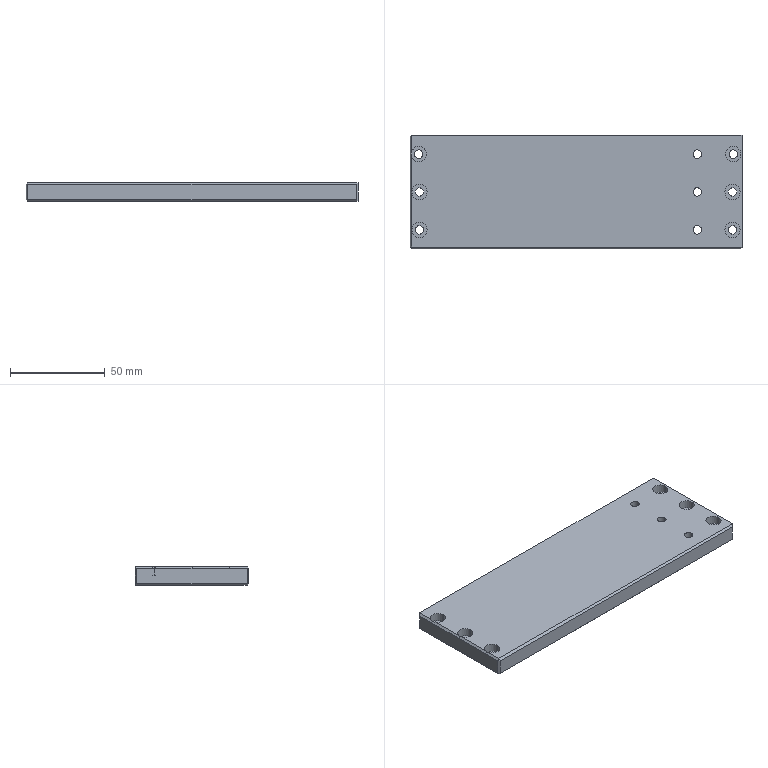Part | STEP file | MT-COMBO-119-S040 | 1 solid | 60 faces | box 175 x 60 x 10 mm | volume 101899 mm3 | cylinder 36 | plane 24 | commonest cylinder face diameters 4.5 x18 8 x18